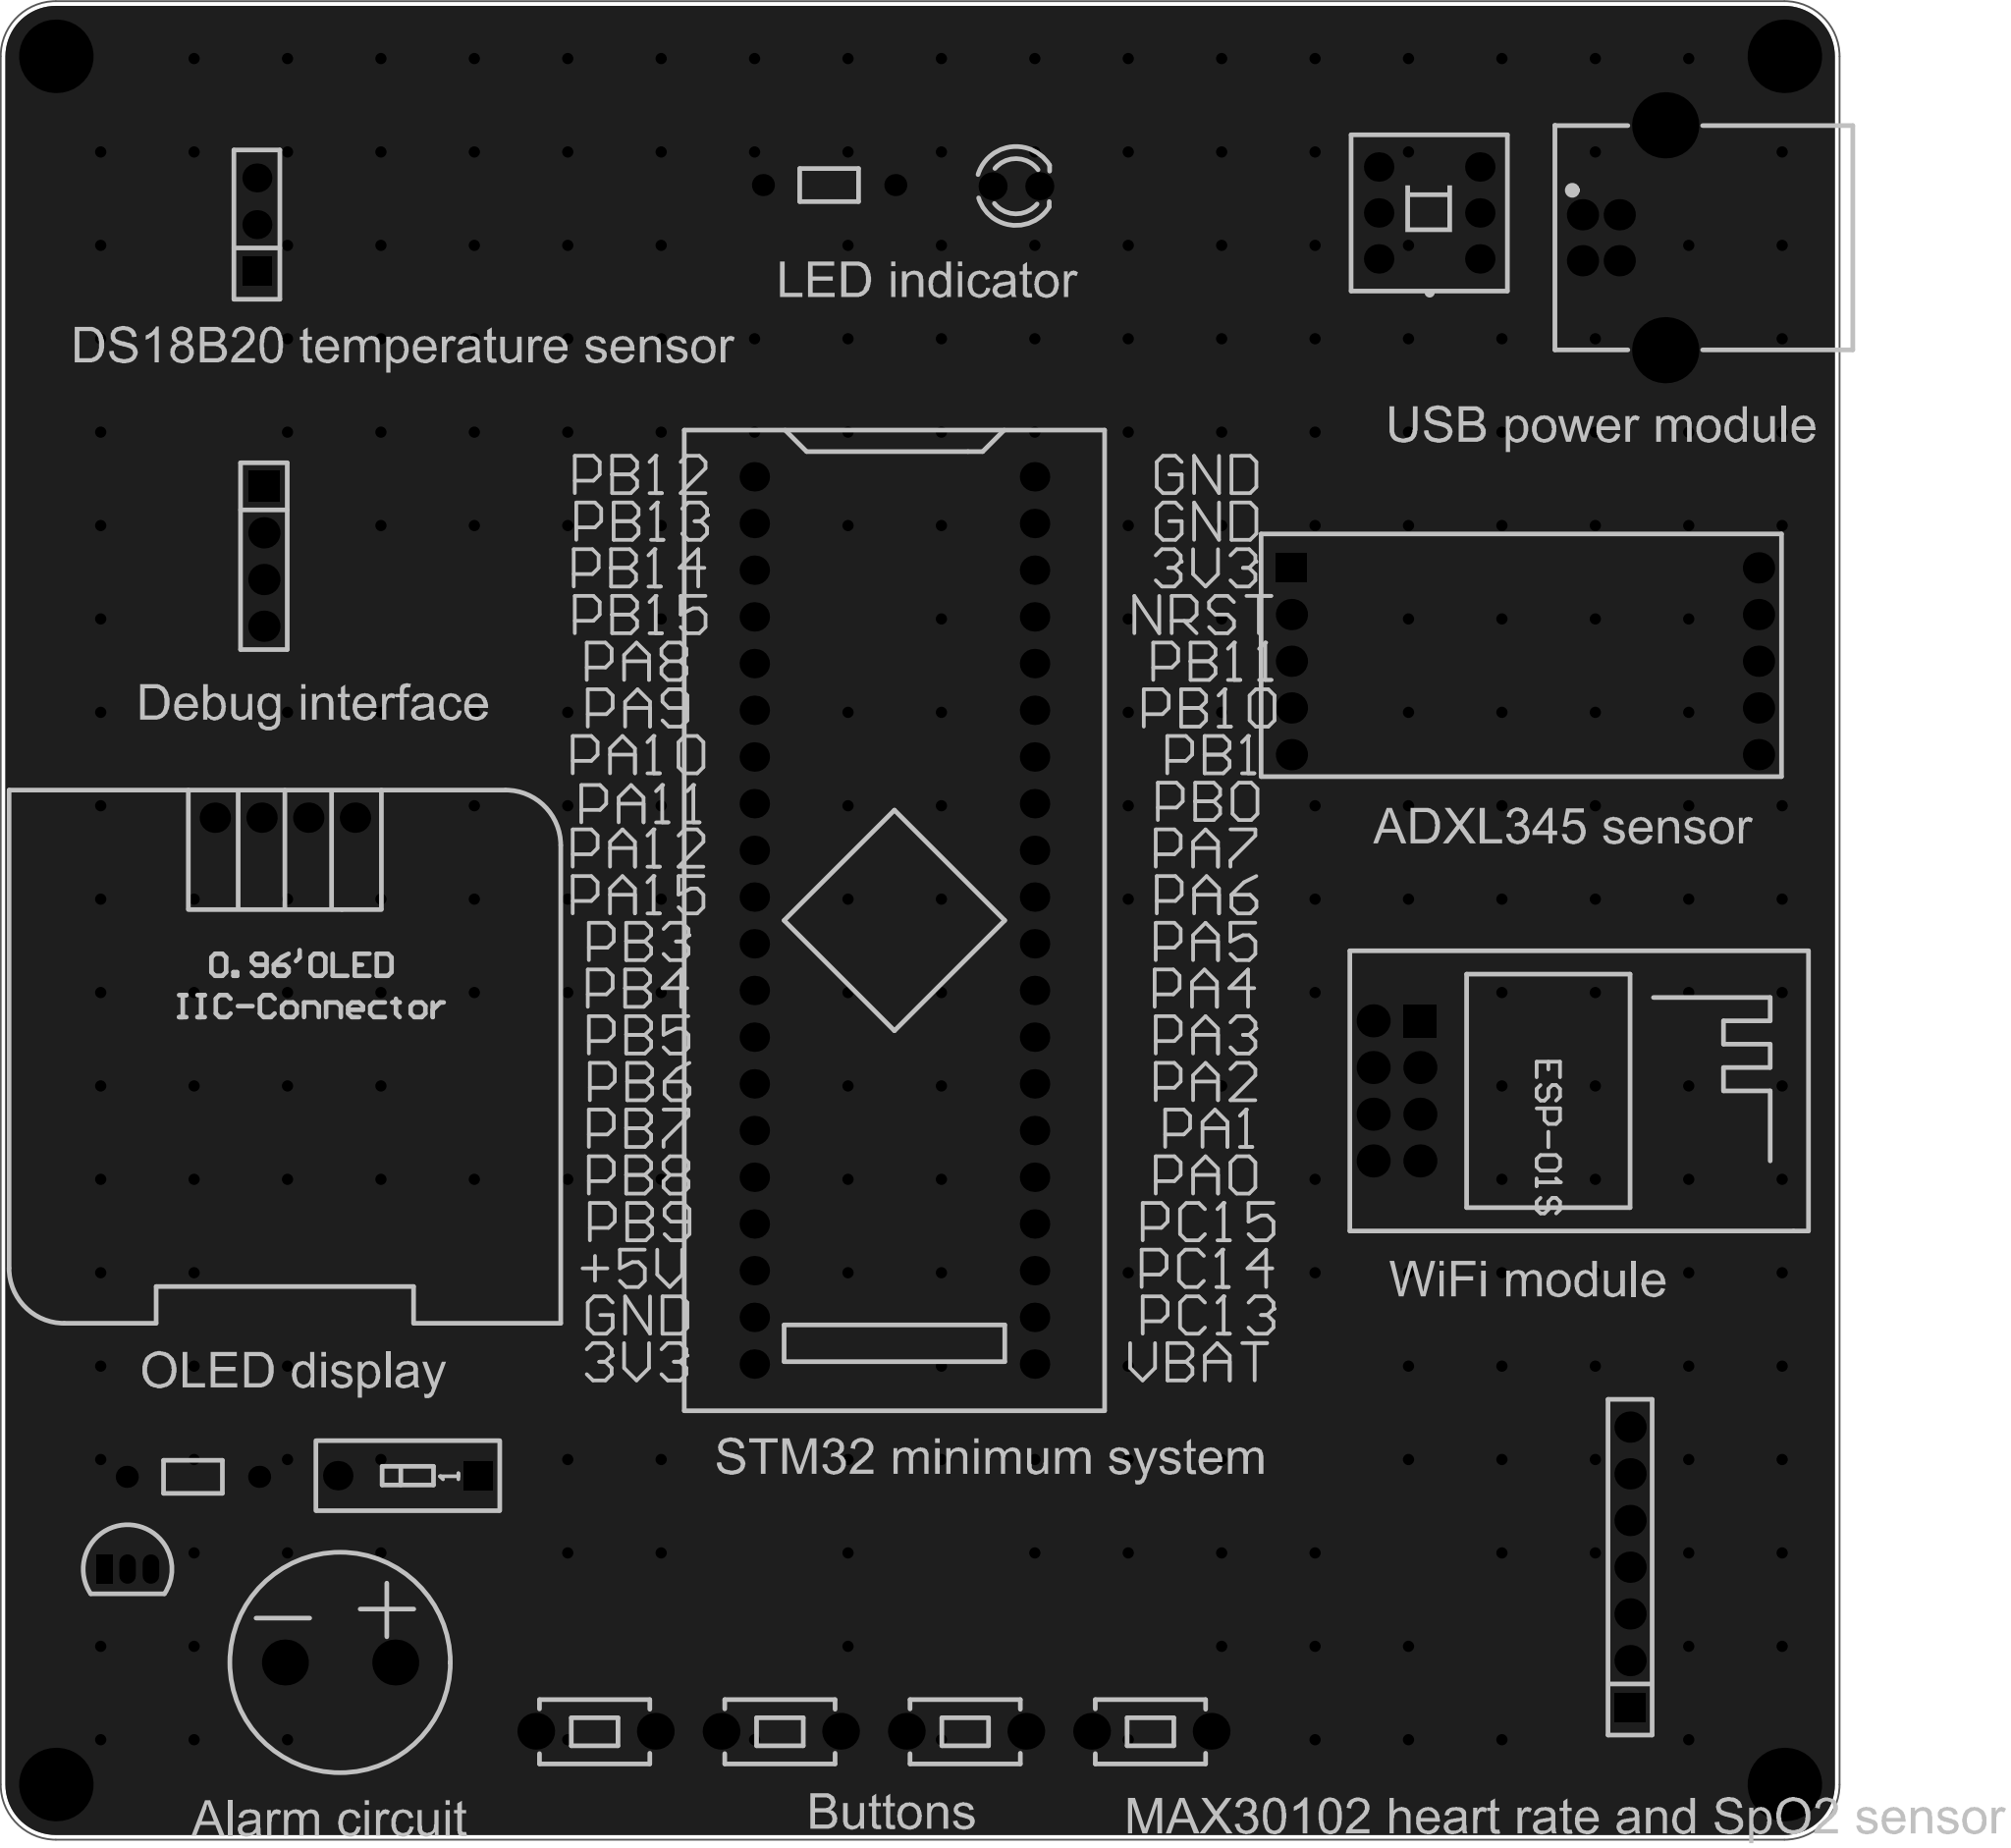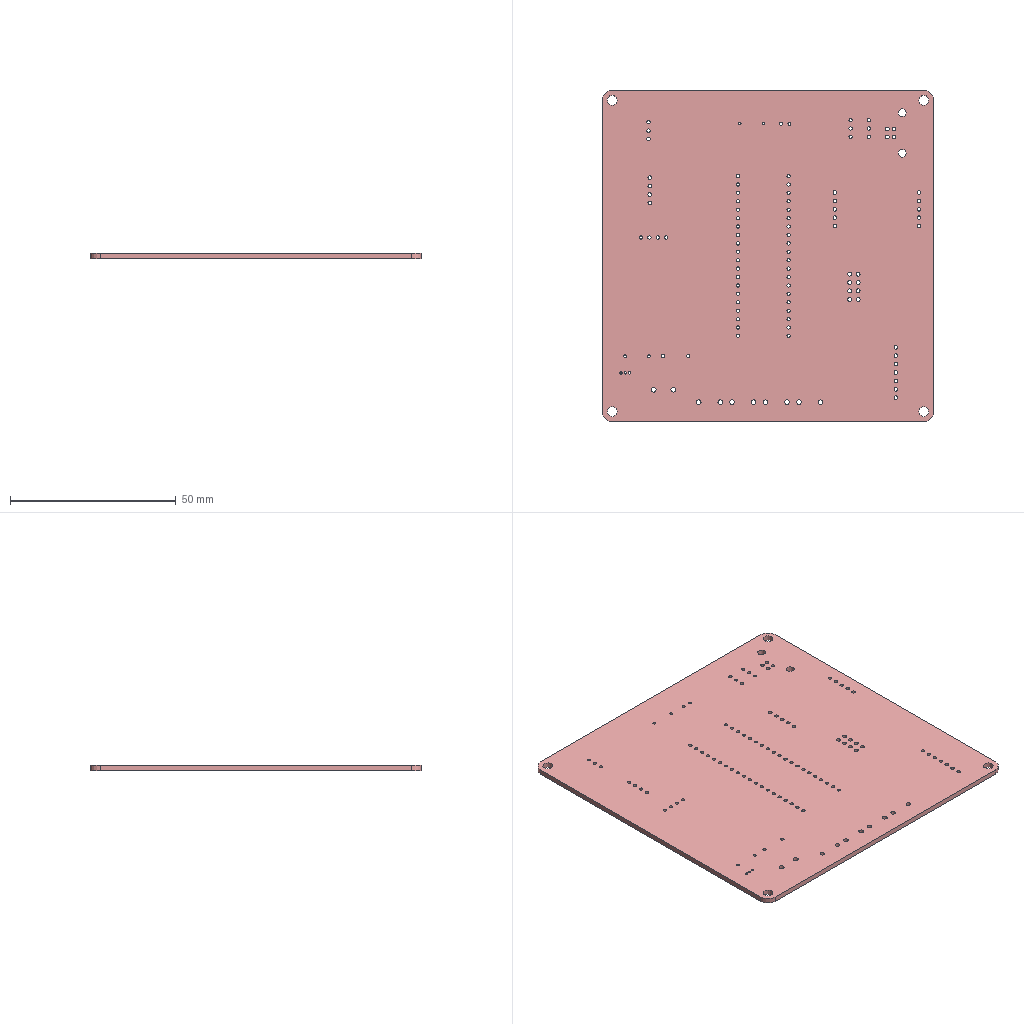Circuit board layout | Altium Designer | box 100 x 100 x 1.6 mm
Layer stack:
# Altium Designer layer stack of  (unit mm; dielectric type: 0 none, 1 core, 2 prepreg, 3 surface material)
index,name,kind,layer,copper_thickness_mm,dielectric_type,dielectric_thickness_mm,dielectric_material,dielectric_constant
0,Top Paste Mask Layer,other,,,,,,
1,Top Silkscreen Layer,other,,,,,,
2,Top Solder Mask Layer,dielectric,,,3,0.01,,3.3
3,Top Layer,copper,Top Layer,0.035,,,,
4,Dielectric1,dielectric,,,3,1.51,FR4,4.5
5,Bottom Layer,copper,Bottom Layer,0.035,,,,
6,Bottom Solder Mask Layer,dielectric,,,3,0.01,,3.3
7,Bottom Silkscreen Layer,other,,,,,,
8,Bottom Paste Mask Layer,other,,,,,,
# drill layer pairs: low layer,high layer
drill_pair,Top Layer,Bottom Layer
Part placement:
Designator,Comment,Layer,Footprint,Center-X(mm),Center-Y(mm),Rotation
U1,STM32F103C8T6-Card,TopLayer,CONN-TH_L53.3-W22.9_STM32F103C8T6-CARD,129.159,128.905,270
BUZZER1,buzzer,TopLayer,BUZ-TH_BD12.0-P6.00-D0.9-RD,99.013,88.545,0
H1,,TopLayer,HDR-TH_4P-P2.54-V-M,94.869,148.717,270
H2,,TopLayer,HDR-TH_10P-P2.54-V-F-R2-C5-S2.54,163.449,143.002,270
H3,,TopLayer,HDR-TH_3P-P2.54-V-F,94.488,166.751,90
H4,,TopLayer,HDR-TH_7P-P2.54-V-F,169.164,93.726,90
KEY1,Non-self-locking switch 8.5×8.5 silent,TopLayer,SW-TH_6P-L8.5-W8.5-P2.54,158.242,167.386,90
LED1,,TopLayer,LED_TH-3mm,135.768,168.839,0
OLED1,,TopLayer,0.96OLED_4P,96.012,134.493,0
Q1,,TopLayer,S8050_TO_92,87.456,93.625,0
R1,220,TopLayer,Res_1/8W,125.608,168.902,0
SW1,,TopLayer,Key_TH_3.5x6x4.3,143.131,84.803,0
SW2,,TopLayer,Key_TH_3.5x6x4.3,133.056,84.803,0
SW3,,TopLayer,Key_TH_3.5x6x4.3,122.981,84.803,0
SW4,,TopLayer,Key_TH_3.5x6x4.3,112.905,84.803,0
SW5,NDS-01V,TopLayer,SW-TH_2P-L3.9-W9.9-P2.54-LS7.6,102.696,98.705,180
U2,ESP-01S,TopLayer,WIFIM-TH_ESP-01S,156.464,119.634,270
USB1,,TopLayer,USB__Type-B,168.827,166.037,90
R2,10kΩ,TopLayer,Res_1/8W,91.012,98.642,180
Pad and via stacks:
# Altium Designer via and pad stacks of  (unit mm). Each distinct definition once, with the count of objects using it.
# via: kind,start_layer,end_layer,hole_mm,diameter_mm,mode(0 simple;1 top-mid-bottom;2 full stack),diameter_per_layer,count,example_net
# pad: kind,layer,hole_mm,hole_type(0 round;1 square;2 slot),plating,top_size,top_shape(1 round;2 rect;3 octagon;9 rounded rect),mid_size,bottom_size,mode,footprint,size_per_layer,count,example
pad,Multi-Layer,3,0,plated,4x4,1,4x4,4x4,0,,,4,1
pad,Multi-Layer,1,0,plated,1.6x1.6,1,1.6x1.6,1.6x1.6,0,CONN-TH_L53.3-W22.9_STM32F103C8T6-CARD,,40,U1.1
pad,Multi-Layer,1.5,0,plated,2.5x2.5,1,2.5x2.5,2.5x2.5,0,BUZ-TH_BD12.0-P6.00-D0.9-RD,,2,BUZZER1.1
pad,Multi-Layer,1.1,0,plated,1.7x1.7,2,1.7x1.7,1.7x1.7,0,HDR-TH_4P-P2.54-V-M,,1,H1.1
pad,Multi-Layer,1.1,0,plated,1.7x1.7,1,1.7x1.7,1.7x1.7,0,HDR-TH_4P-P2.54-V-M,,3,H1.2
pad,Multi-Layer,1.1,0,plated,1.7x1.7,1,1.7x1.7,1.7x1.7,0,HDR-TH_10P-P2.54-V-F-R2-C5-S2.54,,9,H2.10
pad,Multi-Layer,1.1,0,plated,1.575x1.7,2,1.575x1.7,1.575x1.7,0,HDR-TH_10P-P2.54-V-F-R2-C5-S2.54,,1,H2.1
pad,Multi-Layer,1.02,0,plated,1.575x1.575,1,1.575x1.575,1.575x1.575,0,HDR-TH_3P-P2.54-V-F,,2,H3.3
pad,Multi-Layer,1.02,0,plated,1.575x1.575,2,1.575x1.575,1.575x1.575,0,HDR-TH_3P-P2.54-V-F,,1,H3.1
pad,Multi-Layer,1.1,0,plated,1.7x1.7,1,1.7x1.7,1.7x1.7,0,HDR-TH_7P-P2.54-V-F,,6,H4.7
pad,Multi-Layer,1.1,0,plated,1.575x1.7,2,1.575x1.7,1.575x1.7,0,HDR-TH_7P-P2.54-V-F,,1,H4.1
pad,Multi-Layer,1,0,plated,1.6x1.6,1,1.6x1.6,1.6x1.6,0,SW-TH_6P-L8.5-W8.5-P2.54,,6,KEY1.4
pad,Multi-Layer,0.9144,0,plated,1.524x1.524,1,1.524x1.524,1.524x1.524,0,LED_TH-3mm,,2,LED1.1
pad,Multi-Layer,1,0,plated,1.65x1.65,1,1.65x1.65,1.65x1.65,0,0.96OLED_4P,,4,OLED1.4
pad,Multi-Layer,0.701,0,plated,0.8992x1.6,2,0.8992x1.6,0.8992x1.6,0,S8050_TO_92,,1,Q1.1
pad,Multi-Layer,0.701,0,plated,0.8992x1.6,1,0.8992x1.6,0.8992x1.6,0,S8050_TO_92,,2,Q1.2
pad,Multi-Layer,0.8001,0,plated,1.199x1.199,1,1.199x1.199,1.199x1.199,0,Res_1/8W,,4,R1.1
pad,Multi-Layer,1.399,0,plated,1.999x1.999,1,1.999x1.999,1.999x1.999,0,Key_TH_3.5x6x4.3,,8,SW1.A
pad,Multi-Layer,1,0,plated,1.6x1.6,2,1.6x1.6,1.6x1.6,0,SW-TH_2P-L3.9-W9.9-P2.54-LS7.6,,1,SW5.1
pad,Multi-Layer,1,0,plated,1.6x1.6,1,1.6x1.6,1.6x1.6,0,SW-TH_2P-L3.9-W9.9-P2.54-LS7.6,,1,SW5.2
pad,Multi-Layer,1.2,0,plated,1.8x1.8,2,1.8x1.8,1.8x1.8,0,WIFIM-TH_ESP-01S,,1,U2.1
pad,Multi-Layer,1.2,0,plated,1.8x1.8,1,1.8x1.8,1.8x1.8,0,WIFIM-TH_ESP-01S,,7,U2.2
pad,Multi-Layer,1.1,0,plated,1.7x1.7,1,1.7x1.7,1.7x1.7,0,USB_ Type-B,,4,USB1.3
pad,Multi-Layer,2.4,0,plated,3.6x3.6,1,3.6x3.6,3.6x3.6,0,USB_ Type-B,,2,USB1.5
via,Top Layer,Bottom Layer,0.3048,0.61,0,,259,GND
Copper pours:
name,layer,net,type(0 solid;1 hatched;2 none)
Bottom Layer-GND,Bottom Layer,GND,0
Top Layer-GND,Top Layer,GND,0
Design rules, without the lines most boards share:
# Altium Designer design rules of  (exported by Altium Designer, unit mm)
# columns: name | kind | enabled | priority | scope1 | scope2 | descriptor | typed fields (field=value)
copperThickness1oz_2 | 2 | enabled | 2 | All | All | Width Constraint (Min=5mil) (Max=100mil) (Preferred=30mil) (All) |
viaSize | 11 | enabled | 1 | All | All | Routing Via (MinHoleWidth=11.811mil) (MaxHoleWidth=248.032mil) (PreferredHoleWidth=12.008mil) (MinWidth=19.685mil) (MaxWidth=393.701mil) (PreferedWidth=24.016mil) (All) | via_min_hole=0.3 via_max_hole=6.3 via_preferred_diameter=0.61 via_preferred_hole=0.305
solderMaskExpansion | 13 | enabled | 2 | All | All | Solder Mask Expansion (Expansion =2.008mil) (All) | expansion=0.051